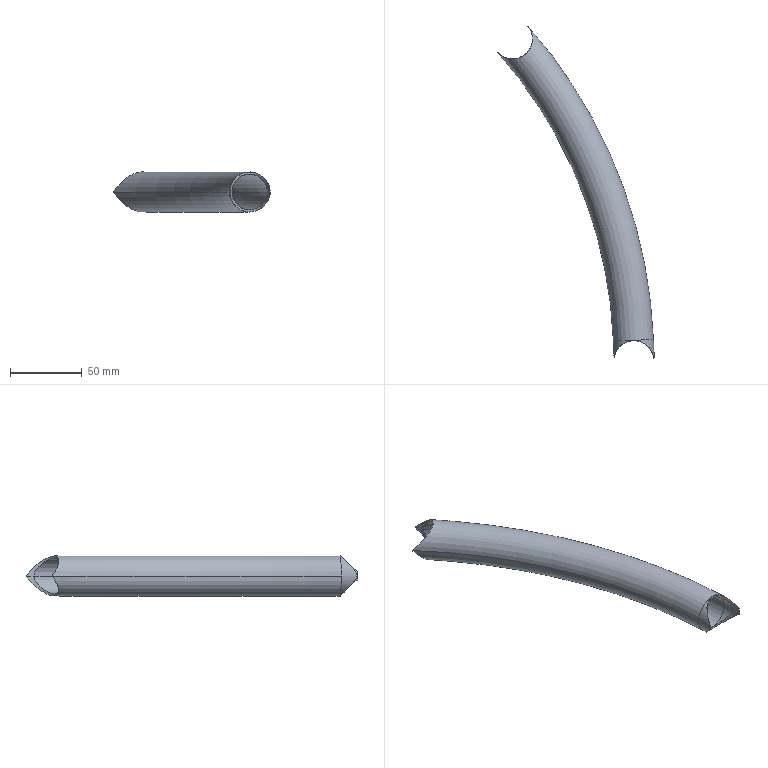Part | STEP file | PRT0001_68_24 | 1 solid | 9 faces | box 109.297 x 231.955 x 28 mm | volume 28262 mm3 | torus 4 | cylinder 3 | plane 1 | cone 1 | commonest cylinder face diameters 25 x1 28 x1 28.01 x1